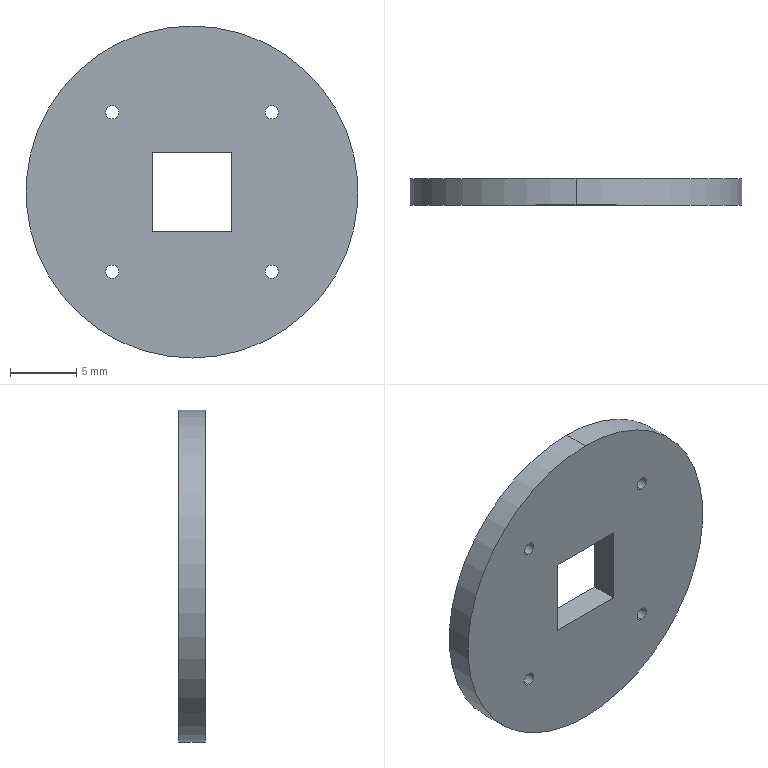Part | SolidWorks | features Extrusion 1 | 1 solid | 16 faces | box 25 x 2 x 25 mm | volume 903.465 mm3 | cylinder 10 | plane 6 | commonest cylinder face diameters 1 x8 25 x2
STEP:
#1=CARTESIAN_POINT('',(6.,2.,5.5));
#2=VERTEX_POINT('',#1);
#3=CARTESIAN_POINT('',(6.,2.,6.5));
#4=VERTEX_POINT('',#3);
#5=CARTESIAN_POINT('',(6.,2.,6.));
#6=DIRECTION('',(0.,1.,0.));
#7=DIRECTION('',(0.,0.,1.));
#8=AXIS2_PLACEMENT_3D('',#5,#6,#7);
#9=CIRCLE('',#8,0.5);
#10=EDGE_CURVE('',#2,#4,#9,.T.);
#11=ORIENTED_EDGE('',*,*,#10,.T.);
#12=CARTESIAN_POINT('',(6.,0.,6.5));
#13=VERTEX_POINT('',#12);
#14=CARTESIAN_POINT('',(6.,2.,6.5));
#15=DIRECTION('',(0.,-1.,0.));
#16=VECTOR('',#15,1000.);
#17=LINE('',#14,#16);
#18=EDGE_CURVE('',#4,#13,#17,.T.);
#19=ORIENTED_EDGE('',*,*,#18,.T.);
#20=CARTESIAN_POINT('',(6.,0.,5.5));
#21=VERTEX_POINT('',#20);
#22=CARTESIAN_POINT('',(6.,0.,6.));
#23=DIRECTION('',(0.,1.,0.));
#24=DIRECTION('',(0.,0.,1.));
#25=AXIS2_PLACEMENT_3D('',#22,#23,#24);
#26=CIRCLE('',#25,0.5);
#27=EDGE_CURVE('',#21,#13,#26,.T.);
#28=ORIENTED_EDGE('',*,*,#27,.F.);
#29=CARTESIAN_POINT('',(6.,2.,5.5));
#30=DIRECTION('',(0.,-1.,0.));
#31=VECTOR('',#30,1000.);
#32=LINE('',#29,#31);
#33=EDGE_CURVE('',#2,#21,#32,.T.);
#34=ORIENTED_EDGE('',*,*,#33,.F.);
#35=EDGE_LOOP('',(#11,#19,#28,#34));
#36=FACE_OUTER_BOUND('',#35,.T.);
#37=CARTESIAN_POINT('',(6.,2.,6.));
#38=DIRECTION('',(0.,-1.,0.));
#39=DIRECTION('',(0.,0.,-1.));
#40=AXIS2_PLACEMENT_3D('',#37,#38,#39);
#41=CYLINDRICAL_SURFACE('',#40,0.5);
#42=ADVANCED_FACE('',(#36),#41,.F.);
#43=CARTESIAN_POINT('',(6.,2.,-6.5));
#44=VERTEX_POINT('',#43);
#45=CARTESIAN_POINT('',(6.,2.,-5.5));
#46=VERTEX_POINT('',#45);
#47=CARTESIAN_POINT('',(6.,2.,-6.));
#48=DIRECTION('',(0.,1.,0.));
#49=DIRECTION('',(0.,0.,1.));
#50=AXIS2_PLACEMENT_3D('',#47,#48,#49);
#51=CIRCLE('',#50,0.5);
#52=EDGE_CURVE('',#44,#46,#51,.T.);
#53=ORIENTED_EDGE('',*,*,#52,.T.);
#54=CARTESIAN_POINT('',(6.,0.,-5.5));
#55=VERTEX_POINT('',#54);
#56=CARTESIAN_POINT('',(6.,2.,-5.5));
#57=DIRECTION('',(0.,-1.,0.));
#58=VECTOR('',#57,1000.);
#59=LINE('',#56,#58);
#60=EDGE_CURVE('',#46,#55,#59,.T.);
#61=ORIENTED_EDGE('',*,*,#60,.T.);
#62=CARTESIAN_POINT('',(6.,0.,-6.5));
#63=VERTEX_POINT('',#62);
#64=CARTESIAN_POINT('',(6.,0.,-6.));
#65=DIRECTION('',(0.,1.,0.));
#66=DIRECTION('',(0.,0.,1.));
#67=AXIS2_PLACEMENT_3D('',#64,#65,#66);
#68=CIRCLE('',#67,0.5);
#69=EDGE_CURVE('',#63,#55,#68,.T.);
#70=ORIENTED_EDGE('',*,*,#69,.F.);
#71=CARTESIAN_POINT('',(6.,2.,-6.5));
#72=DIRECTION('',(0.,-1.,0.));
#73=VECTOR('',#72,1000.);
#74=LINE('',#71,#73);
#75=EDGE_CURVE('',#44,#63,#74,.T.);
#76=ORIENTED_EDGE('',*,*,#75,.F.);
#77=EDGE_LOOP('',(#53,#61,#70,#76));
#78=FACE_OUTER_BOUND('',#77,.T.);
#79=CARTESIAN_POINT('',(6.,2.,-6.));
#80=DIRECTION('',(0.,-1.,0.));
#81=DIRECTION('',(0.,0.,-1.));
#82=AXIS2_PLACEMENT_3D('',#79,#80,#81);
#83=CYLINDRICAL_SURFACE('',#82,0.5);
#84=ADVANCED_FACE('',(#78),#83,.F.);
#85=CARTESIAN_POINT('',(-6.,2.,5.5));
#86=VERTEX_POINT('',#85);
#87=CARTESIAN_POINT('',(-6.,2.,6.5));
#88=VERTEX_POINT('',#87);
#89=CARTESIAN_POINT('',(-6.,2.,6.));
#90=DIRECTION('',(0.,1.,0.));
#91=DIRECTION('',(0.,0.,1.));
#92=AXIS2_PLACEMENT_3D('',#89,#90,#91);
#93=CIRCLE('',#92,0.5);
#94=EDGE_CURVE('',#86,#88,#93,.T.);
#95=ORIENTED_EDGE('',*,*,#94,.T.);
#96=CARTESIAN_POINT('',(-6.,0.,6.5));
#97=VERTEX_POINT('',#96);
#98=CARTESIAN_POINT('',(-6.,2.,6.5));
#99=DIRECTION('',(0.,-1.,0.));
#100=VECTOR('',#99,1000.);
#101=LINE('',#98,#100);
#102=EDGE_CURVE('',#88,#97,#101,.T.);
#103=ORIENTED_EDGE('',*,*,#102,.T.);
#104=CARTESIAN_POINT('',(-6.,0.,5.5));
#105=VERTEX_POINT('',#104);
#106=CARTESIAN_POINT('',(-6.,0.,6.));
#107=DIRECTION('',(0.,1.,0.));
#108=DIRECTION('',(0.,0.,1.));
#109=AXIS2_PLACEMENT_3D('',#106,#107,#108);
#110=CIRCLE('',#109,0.5);
#111=EDGE_CURVE('',#105,#97,#110,.T.);
#112=ORIENTED_EDGE('',*,*,#111,.F.);
#113=CARTESIAN_POINT('',(-6.,2.,5.5));
#114=DIRECTION('',(0.,-1.,0.));
#115=VECTOR('',#114,1000.);
#116=LINE('',#113,#115);
#117=EDGE_CURVE('',#86,#105,#116,.T.);
#118=ORIENTED_EDGE('',*,*,#117,.F.);
#119=EDGE_LOOP('',(#95,#103,#112,#118));
#120=FACE_OUTER_BOUND('',#119,.T.);
#121=CARTESIAN_POINT('',(-6.,2.,6.));
#122=DIRECTION('',(0.,-1.,0.));
#123=DIRECTION('',(0.,0.,-1.));
#124=AXIS2_PLACEMENT_3D('',#121,#122,#123);
#125=CYLINDRICAL_SURFACE('',#124,0.5);
#126=ADVANCED_FACE('',(#120),#125,.F.);
#127=CARTESIAN_POINT('',(-6.,2.,-6.5));
#128=VERTEX_POINT('',#127);
#129=CARTESIAN_POINT('',(-6.,2.,-5.5));
#130=VERTEX_POINT('',#129);
#131=CARTESIAN_POINT('',(-6.,2.,-6.));
#132=DIRECTION('',(0.,1.,0.));
#133=DIRECTION('',(0.,0.,1.));
#134=AXIS2_PLACEMENT_3D('',#131,#132,#133);
#135=CIRCLE('',#134,0.5);
#136=EDGE_CURVE('',#128,#130,#135,.T.);
#137=ORIENTED_EDGE('',*,*,#136,.T.);
#138=CARTESIAN_POINT('',(-6.,0.,-5.5));
#139=VERTEX_POINT('',#138);
#140=CARTESIAN_POINT('',(-6.,2.,-5.5));
#141=DIRECTION('',(0.,-1.,0.));
#142=VECTOR('',#141,1000.);
#143=LINE('',#140,#142);
#144=EDGE_CURVE('',#130,#139,#143,.T.);
#145=ORIENTED_EDGE('',*,*,#144,.T.);
#146=CARTESIAN_POINT('',(-6.,0.,-6.5));
#147=VERTEX_POINT('',#146);
#148=CARTESIAN_POINT('',(-6.,0.,-6.));
#149=DIRECTION('',(0.,1.,0.));
#150=DIRECTION('',(0.,0.,1.));
#151=AXIS2_PLACEMENT_3D('',#148,#149,#150);
#152=CIRCLE('',#151,0.5);
#153=EDGE_CURVE('',#147,#139,#152,.T.);
#154=ORIENTED_EDGE('',*,*,#153,.F.);
#155=CARTESIAN_POINT('',(-6.,2.,-6.5));
#156=DIRECTION('',(0.,-1.,0.));
#157=VECTOR('',#156,1000.);
#158=LINE('',#155,#157);
#159=EDGE_CURVE('',#128,#147,#158,.T.);
#160=ORIENTED_EDGE('',*,*,#159,.F.);
#161=EDGE_LOOP('',(#137,#145,#154,#160));
#162=FACE_OUTER_BOUND('',#161,.T.);
#163=CARTESIAN_POINT('',(-6.,2.,-6.));
#164=DIRECTION('',(0.,-1.,0.));
#165=DIRECTION('',(0.,0.,-1.));
#166=AXIS2_PLACEMENT_3D('',#163,#164,#165);
#167=CYLINDRICAL_SURFACE('',#166,0.5);
#168=ADVANCED_FACE('',(#162),#167,.F.);
#169=CARTESIAN_POINT('',(0.,2.,12.5));
#170=VERTEX_POINT('',#169);
#171=CARTESIAN_POINT('',(0.,2.,-12.5));
#172=VERTEX_POINT('',#171);
#173=CARTESIAN_POINT('',(0.,2.,0.));
#174=DIRECTION('',(0.,1.,0.));
#175=DIRECTION('',(0.,0.,1.));
#176=AXIS2_PLACEMENT_3D('',#173,#174,#175);
#177=CIRCLE('',#176,12.5);
#178=EDGE_CURVE('',#170,#172,#177,.T.);
#179=ORIENTED_EDGE('',*,*,#178,.F.);
#180=CARTESIAN_POINT('',(0.,0.,12.5));
#181=VERTEX_POINT('',#180);
#182=CARTESIAN_POINT('',(0.,2.,12.5));
#183=DIRECTION('',(0.,-1.,0.));
#184=VECTOR('',#183,1000.);
#185=LINE('',#182,#184);
#186=EDGE_CURVE('',#170,#181,#185,.T.);
#187=ORIENTED_EDGE('',*,*,#186,.T.);
#188=CARTESIAN_POINT('',(0.,0.,-12.5));
#189=VERTEX_POINT('',#188);
#190=CARTESIAN_POINT('',(0.,0.,0.));
#191=DIRECTION('',(0.,1.,0.));
#192=DIRECTION('',(0.,0.,1.));
#193=AXIS2_PLACEMENT_3D('',#190,#191,#192);
#194=CIRCLE('',#193,12.5);
#195=EDGE_CURVE('',#181,#189,#194,.T.);
#196=ORIENTED_EDGE('',*,*,#195,.T.);
#197=CARTESIAN_POINT('',(0.,2.,-12.5));
#198=DIRECTION('',(0.,-1.,0.));
#199=VECTOR('',#198,1000.);
#200=LINE('',#197,#199);
#201=EDGE_CURVE('',#172,#189,#200,.T.);
#202=ORIENTED_EDGE('',*,*,#201,.F.);
#203=EDGE_LOOP('',(#179,#187,#196,#202));
#204=FACE_OUTER_BOUND('',#203,.T.);
#205=CARTESIAN_POINT('',(0.,2.,0.));
#206=DIRECTION('',(0.,-1.,0.));
#207=DIRECTION('',(0.,0.,-1.));
#208=AXIS2_PLACEMENT_3D('',#205,#206,#207);
#209=CYLINDRICAL_SURFACE('',#208,12.5);
#210=ADVANCED_FACE('',(#204),#209,.T.);
#211=ORIENTED_EDGE('',*,*,#52,.F.);
#212=CARTESIAN_POINT('',(6.,2.,-6.));
#213=DIRECTION('',(0.,1.,0.));
#214=DIRECTION('',(0.,0.,1.));
#215=AXIS2_PLACEMENT_3D('',#212,#213,#214);
#216=CIRCLE('',#215,0.5);
#217=EDGE_CURVE('',#46,#44,#216,.T.);
#218=ORIENTED_EDGE('',*,*,#217,.F.);
#219=EDGE_LOOP('',(#211,#218));
#220=FACE_BOUND('',#219,.T.);
#221=ORIENTED_EDGE('',*,*,#136,.F.);
#222=CARTESIAN_POINT('',(-6.,2.,-6.));
#223=DIRECTION('',(0.,1.,0.));
#224=DIRECTION('',(0.,0.,1.));
#225=AXIS2_PLACEMENT_3D('',#222,#223,#224);
#226=CIRCLE('',#225,0.5);
#227=EDGE_CURVE('',#130,#128,#226,.T.);
#228=ORIENTED_EDGE('',*,*,#227,.F.);
#229=EDGE_LOOP('',(#221,#228));
#230=FACE_BOUND('',#229,.T.);
#231=CARTESIAN_POINT('',(0.,2.,0.));
#232=DIRECTION('',(0.,1.,0.));
#233=DIRECTION('',(0.,0.,1.));
#234=AXIS2_PLACEMENT_3D('',#231,#232,#233);
#235=CIRCLE('',#234,12.5);
#236=EDGE_CURVE('',#172,#170,#235,.T.);
#237=ORIENTED_EDGE('',*,*,#236,.T.);
#238=ORIENTED_EDGE('',*,*,#178,.T.);
#239=EDGE_LOOP('',(#237,#238));
#240=FACE_OUTER_BOUND('',#239,.T.);
#241=CARTESIAN_POINT('',(3.,2.,-3.));
#242=VERTEX_POINT('',#241);
#243=CARTESIAN_POINT('',(-3.,2.,-3.));
#244=VERTEX_POINT('',#243);
#245=CARTESIAN_POINT('',(3.,2.,-3.));
#246=DIRECTION('',(-1.,0.,0.));
#247=VECTOR('',#246,1000.);
#248=LINE('',#245,#247);
#249=EDGE_CURVE('',#242,#244,#248,.T.);
#250=ORIENTED_EDGE('',*,*,#249,.F.);
#251=CARTESIAN_POINT('',(3.,2.,3.));
#252=VERTEX_POINT('',#251);
#253=CARTESIAN_POINT('',(3.,2.,3.));
#254=DIRECTION('',(0.,0.,-1.));
#255=VECTOR('',#254,1000.);
#256=LINE('',#253,#255);
#257=EDGE_CURVE('',#252,#242,#256,.T.);
#258=ORIENTED_EDGE('',*,*,#257,.F.);
#259=CARTESIAN_POINT('',(-3.,2.,3.));
#260=VERTEX_POINT('',#259);
#261=CARTESIAN_POINT('',(-3.,2.,3.));
#262=DIRECTION('',(1.,0.,0.));
#263=VECTOR('',#262,1000.);
#264=LINE('',#261,#263);
#265=EDGE_CURVE('',#260,#252,#264,.T.);
#266=ORIENTED_EDGE('',*,*,#265,.F.);
#267=CARTESIAN_POINT('',(-3.,2.,-3.));
#268=DIRECTION('',(0.,0.,1.));
#269=VECTOR('',#268,1000.);
#270=LINE('',#267,#269);
#271=EDGE_CURVE('',#244,#260,#270,.T.);
#272=ORIENTED_EDGE('',*,*,#271,.F.);
#273=EDGE_LOOP('',(#250,#258,#266,#272));
#274=FACE_BOUND('',#273,.T.);
#275=ORIENTED_EDGE('',*,*,#94,.F.);
#276=CARTESIAN_POINT('',(-6.,2.,6.));
#277=DIRECTION('',(0.,1.,0.));
#278=DIRECTION('',(0.,0.,1.));
#279=AXIS2_PLACEMENT_3D('',#276,#277,#278);
#280=CIRCLE('',#279,0.5);
#281=EDGE_CURVE('',#88,#86,#280,.T.);
#282=ORIENTED_EDGE('',*,*,#281,.F.);
#283=EDGE_LOOP('',(#275,#282));
#284=FACE_BOUND('',#283,.T.);
#285=ORIENTED_EDGE('',*,*,#10,.F.);
#286=CARTESIAN_POINT('',(6.,2.,6.));
#287=DIRECTION('',(0.,1.,0.));
#288=DIRECTION('',(0.,0.,1.));
#289=AXIS2_PLACEMENT_3D('',#286,#287,#288);
#290=CIRCLE('',#289,0.5);
#291=EDGE_CURVE('',#4,#2,#290,.T.);
#292=ORIENTED_EDGE('',*,*,#291,.F.);
#293=EDGE_LOOP('',(#285,#292));
#294=FACE_BOUND('',#293,.T.);
#295=CARTESIAN_POINT('',(0.,2.,0.));
#296=DIRECTION('',(0.,1.,0.));
#297=DIRECTION('',(0.,0.,1.));
#298=AXIS2_PLACEMENT_3D('',#295,#296,#297);
#299=PLANE('',#298);
#300=ADVANCED_FACE('',(#220,#230,#240,#274,#284,#294),#299,.T.);
#301=CARTESIAN_POINT('',(0.,0.,0.));
#302=DIRECTION('',(0.,1.,0.));
#303=DIRECTION('',(0.,0.,1.));
#304=AXIS2_PLACEMENT_3D('',#301,#302,#303);
#305=CIRCLE('',#304,12.5);
#306=EDGE_CURVE('',#189,#181,#305,.T.);
#307=ORIENTED_EDGE('',*,*,#306,.F.);
#308=ORIENTED_EDGE('',*,*,#195,.F.);
#309=EDGE_LOOP('',(#307,#308));
#310=FACE_OUTER_BOUND('',#309,.T.);
#311=CARTESIAN_POINT('',(3.,0.,3.));
#312=VERTEX_POINT('',#311);
#313=CARTESIAN_POINT('',(3.,0.,-3.));
#314=VERTEX_POINT('',#313);
#315=CARTESIAN_POINT('',(3.,0.,3.));
#316=DIRECTION('',(0.,0.,-1.));
#317=VECTOR('',#316,1000.);
#318=LINE('',#315,#317);
#319=EDGE_CURVE('',#312,#314,#318,.T.);
#320=ORIENTED_EDGE('',*,*,#319,.T.);
#321=CARTESIAN_POINT('',(-3.,0.,-3.));
#322=VERTEX_POINT('',#321);
#323=CARTESIAN_POINT('',(3.,0.,-3.));
#324=DIRECTION('',(-1.,0.,0.));
#325=VECTOR('',#324,1000.);
#326=LINE('',#323,#325);
#327=EDGE_CURVE('',#314,#322,#326,.T.);
#328=ORIENTED_EDGE('',*,*,#327,.T.);
#329=CARTESIAN_POINT('',(-3.,0.,3.));
#330=VERTEX_POINT('',#329);
#331=CARTESIAN_POINT('',(-3.,0.,-3.));
#332=DIRECTION('',(0.,0.,1.));
#333=VECTOR('',#332,1000.);
#334=LINE('',#331,#333);
#335=EDGE_CURVE('',#322,#330,#334,.T.);
#336=ORIENTED_EDGE('',*,*,#335,.T.);
#337=CARTESIAN_POINT('',(-3.,0.,3.));
#338=DIRECTION('',(1.,0.,0.));
#339=VECTOR('',#338,1000.);
#340=LINE('',#337,#339);
#341=EDGE_CURVE('',#330,#312,#340,.T.);
#342=ORIENTED_EDGE('',*,*,#341,.T.);
#343=EDGE_LOOP('',(#320,#328,#336,#342));
#344=FACE_BOUND('',#343,.T.);
#345=ORIENTED_EDGE('',*,*,#153,.T.);
#346=CARTESIAN_POINT('',(-6.,0.,-6.));
#347=DIRECTION('',(0.,1.,0.));
#348=DIRECTION('',(0.,0.,1.));
#349=AXIS2_PLACEMENT_3D('',#346,#347,#348);
#350=CIRCLE('',#349,0.5);
#351=EDGE_CURVE('',#139,#147,#350,.T.);
#352=ORIENTED_EDGE('',*,*,#351,.T.);
#353=EDGE_LOOP('',(#345,#352));
#354=FACE_BOUND('',#353,.T.);
#355=ORIENTED_EDGE('',*,*,#111,.T.);
#356=CARTESIAN_POINT('',(-6.,0.,6.));
#357=DIRECTION('',(0.,1.,0.));
#358=DIRECTION('',(0.,0.,1.));
#359=AXIS2_PLACEMENT_3D('',#356,#357,#358);
#360=CIRCLE('',#359,0.5);
#361=EDGE_CURVE('',#97,#105,#360,.T.);
#362=ORIENTED_EDGE('',*,*,#361,.T.);
#363=EDGE_LOOP('',(#355,#362));
#364=FACE_BOUND('',#363,.T.);
#365=ORIENTED_EDGE('',*,*,#69,.T.);
#366=CARTESIAN_POINT('',(6.,0.,-6.));
#367=DIRECTION('',(0.,1.,0.));
#368=DIRECTION('',(0.,0.,1.));
#369=AXIS2_PLACEMENT_3D('',#366,#367,#368);
#370=CIRCLE('',#369,0.5);
#371=EDGE_CURVE('',#55,#63,#370,.T.);
#372=ORIENTED_EDGE('',*,*,#371,.T.);
#373=EDGE_LOOP('',(#365,#372));
#374=FACE_BOUND('',#373,.T.);
#375=ORIENTED_EDGE('',*,*,#27,.T.);
#376=CARTESIAN_POINT('',(6.,0.,6.));
#377=DIRECTION('',(0.,1.,0.));
#378=DIRECTION('',(0.,0.,1.));
#379=AXIS2_PLACEMENT_3D('',#376,#377,#378);
#380=CIRCLE('',#379,0.5);
#381=EDGE_CURVE('',#13,#21,#380,.T.);
#382=ORIENTED_EDGE('',*,*,#381,.T.);
#383=EDGE_LOOP('',(#375,#382));
#384=FACE_BOUND('',#383,.T.);
#385=CARTESIAN_POINT('',(0.,0.,0.));
#386=DIRECTION('',(0.,1.,0.));
#387=DIRECTION('',(0.,0.,1.));
#388=AXIS2_PLACEMENT_3D('',#385,#386,#387);
#389=PLANE('',#388);
#390=ADVANCED_FACE('',(#310,#344,#354,#364,#374,#384),#389,.F.);
#391=ORIENTED_EDGE('',*,*,#186,.F.);
#392=ORIENTED_EDGE('',*,*,#236,.F.);
#393=ORIENTED_EDGE('',*,*,#201,.T.);
#394=ORIENTED_EDGE('',*,*,#306,.T.);
#395=EDGE_LOOP('',(#391,#392,#393,#394));
#396=FACE_OUTER_BOUND('',#395,.T.);
#397=CARTESIAN_POINT('',(0.,2.,0.));
#398=DIRECTION('',(0.,-1.,0.));
#399=DIRECTION('',(0.,0.,-1.));
#400=AXIS2_PLACEMENT_3D('',#397,#398,#399);
#401=CYLINDRICAL_SURFACE('',#400,12.5);
#402=ADVANCED_FACE('',(#396),#401,.T.);
#403=ORIENTED_EDGE('',*,*,#319,.F.);
#404=CARTESIAN_POINT('',(3.,2.,3.));
#405=DIRECTION('',(0.,-1.,0.));
#406=VECTOR('',#405,1000.);
#407=LINE('',#404,#406);
#408=EDGE_CURVE('',#252,#312,#407,.T.);
#409=ORIENTED_EDGE('',*,*,#408,.F.);
#410=ORIENTED_EDGE('',*,*,#257,.T.);
#411=CARTESIAN_POINT('',(3.,2.,-3.));
#412=DIRECTION('',(0.,-1.,0.));
#413=VECTOR('',#412,1000.);
#414=LINE('',#411,#413);
#415=EDGE_CURVE('',#242,#314,#414,.T.);
#416=ORIENTED_EDGE('',*,*,#415,.T.);
#417=EDGE_LOOP('',(#403,#409,#410,#416));
#418=FACE_OUTER_BOUND('',#417,.T.);
#419=CARTESIAN_POINT('',(3.,2.,3.));
#420=DIRECTION('',(-1.,0.,0.));
#421=DIRECTION('',(0.,0.,1.));
#422=AXIS2_PLACEMENT_3D('',#419,#420,#421);
#423=PLANE('',#422);
#424=ADVANCED_FACE('',(#418),#423,.T.);
#425=ORIENTED_EDGE('',*,*,#327,.F.);
#426=ORIENTED_EDGE('',*,*,#415,.F.);
#427=ORIENTED_EDGE('',*,*,#249,.T.);
#428=CARTESIAN_POINT('',(-3.,2.,-3.));
#429=DIRECTION('',(0.,-1.,0.));
#430=VECTOR('',#429,1000.);
#431=LINE('',#428,#430);
#432=EDGE_CURVE('',#244,#322,#431,.T.);
#433=ORIENTED_EDGE('',*,*,#432,.T.);
#434=EDGE_LOOP('',(#425,#426,#427,#433));
#435=FACE_OUTER_BOUND('',#434,.T.);
#436=CARTESIAN_POINT('',(3.,2.,-3.));
#437=DIRECTION('',(0.,0.,1.));
#438=DIRECTION('',(1.,0.,0.));
#439=AXIS2_PLACEMENT_3D('',#436,#437,#438);
#440=PLANE('',#439);
#441=ADVANCED_FACE('',(#435),#440,.T.);
#442=ORIENTED_EDGE('',*,*,#335,.F.);
#443=ORIENTED_EDGE('',*,*,#432,.F.);
#444=ORIENTED_EDGE('',*,*,#271,.T.);
#445=CARTESIAN_POINT('',(-3.,2.,3.));
#446=DIRECTION('',(0.,-1.,0.));
#447=VECTOR('',#446,1000.);
#448=LINE('',#445,#447);
#449=EDGE_CURVE('',#260,#330,#448,.T.);
#450=ORIENTED_EDGE('',*,*,#449,.T.);
#451=EDGE_LOOP('',(#442,#443,#444,#450));
#452=FACE_OUTER_BOUND('',#451,.T.);
#453=CARTESIAN_POINT('',(-3.,2.,-3.));
#454=DIRECTION('',(1.,0.,0.));
#455=DIRECTION('',(0.,0.,-1.));
#456=AXIS2_PLACEMENT_3D('',#453,#454,#455);
#457=PLANE('',#456);
#458=ADVANCED_FACE('',(#452),#457,.T.);
#459=ORIENTED_EDGE('',*,*,#341,.F.);
#460=ORIENTED_EDGE('',*,*,#449,.F.);
#461=ORIENTED_EDGE('',*,*,#265,.T.);
#462=ORIENTED_EDGE('',*,*,#408,.T.);
#463=EDGE_LOOP('',(#459,#460,#461,#462));
#464=FACE_OUTER_BOUND('',#463,.T.);
#465=CARTESIAN_POINT('',(-3.,2.,3.));
#466=DIRECTION('',(0.,0.,-1.));
#467=DIRECTION('',(-1.,0.,0.));
#468=AXIS2_PLACEMENT_3D('',#465,#466,#467);
#469=PLANE('',#468);
#470=ADVANCED_FACE('',(#464),#469,.T.);
#471=ORIENTED_EDGE('',*,*,#144,.F.);
#472=ORIENTED_EDGE('',*,*,#227,.T.);
#473=ORIENTED_EDGE('',*,*,#159,.T.);
#474=ORIENTED_EDGE('',*,*,#351,.F.);
#475=EDGE_LOOP('',(#471,#472,#473,#474));
#476=FACE_OUTER_BOUND('',#475,.T.);
#477=CARTESIAN_POINT('',(-6.,2.,-6.));
#478=DIRECTION('',(0.,-1.,0.));
#479=DIRECTION('',(0.,0.,-1.));
#480=AXIS2_PLACEMENT_3D('',#477,#478,#479);
#481=CYLINDRICAL_SURFACE('',#480,0.5);
#482=ADVANCED_FACE('',(#476),#481,.F.);
#483=ORIENTED_EDGE('',*,*,#102,.F.);
#484=ORIENTED_EDGE('',*,*,#281,.T.);
#485=ORIENTED_EDGE('',*,*,#117,.T.);
#486=ORIENTED_EDGE('',*,*,#361,.F.);
#487=EDGE_LOOP('',(#483,#484,#485,#486));
#488=FACE_OUTER_BOUND('',#487,.T.);
#489=CARTESIAN_POINT('',(-6.,2.,6.));
#490=DIRECTION('',(0.,-1.,0.));
#491=DIRECTION('',(0.,0.,-1.));
#492=AXIS2_PLACEMENT_3D('',#489,#490,#491);
#493=CYLINDRICAL_SURFACE('',#492,0.5);
#494=ADVANCED_FACE('',(#488),#493,.F.);
#495=ORIENTED_EDGE('',*,*,#60,.F.);
#496=ORIENTED_EDGE('',*,*,#217,.T.);
#497=ORIENTED_EDGE('',*,*,#75,.T.);
#498=ORIENTED_EDGE('',*,*,#371,.F.);
#499=EDGE_LOOP('',(#495,#496,#497,#498));
#500=FACE_OUTER_BOUND('',#499,.T.);
#501=CARTESIAN_POINT('',(6.,2.,-6.));
#502=DIRECTION('',(0.,-1.,0.));
#503=DIRECTION('',(0.,0.,-1.));
#504=AXIS2_PLACEMENT_3D('',#501,#502,#503);
#505=CYLINDRICAL_SURFACE('',#504,0.5);
#506=ADVANCED_FACE('',(#500),#505,.F.);
#507=ORIENTED_EDGE('',*,*,#18,.F.);
#508=ORIENTED_EDGE('',*,*,#291,.T.);
#509=ORIENTED_EDGE('',*,*,#33,.T.);
#510=ORIENTED_EDGE('',*,*,#381,.F.);
#511=EDGE_LOOP('',(#507,#508,#509,#510));
#512=FACE_OUTER_BOUND('',#511,.T.);
#513=CARTESIAN_POINT('',(6.,2.,6.));
#514=DIRECTION('',(0.,-1.,0.));
#515=DIRECTION('',(0.,0.,-1.));
#516=AXIS2_PLACEMENT_3D('',#513,#514,#515);
#517=CYLINDRICAL_SURFACE('',#516,0.5);
#518=ADVANCED_FACE('',(#512),#517,.F.);
#519=CLOSED_SHELL('',(#42,#84,#126,#168,#210,#300,#390,#402,#424,#441,#458,#470,#482,#494,#506,#518));
#520=MANIFOLD_SOLID_BREP('',#519);
#521=CARTESIAN_POINT('',(0.,0.,0.));
#522=DIRECTION('',(0.,0.,1.));
#523=DIRECTION('',(1.,0.,0.));
#524=AXIS2_PLACEMENT_3D('',#521,#522,#523);
#525=(LENGTH_UNIT()NAMED_UNIT(*)SI_UNIT(.MILLI.,.METRE.));
#526=UNCERTAINTY_MEASURE_WITH_UNIT(LENGTH_MEASURE(0.00001),#525,'','');
#527=(NAMED_UNIT(*)PLANE_ANGLE_UNIT()SI_UNIT($,.RADIAN.));
#528=(NAMED_UNIT(*)SI_UNIT($,.STERADIAN.)SOLID_ANGLE_UNIT());
#529=(GEOMETRIC_REPRESENTATION_CONTEXT(3)GLOBAL_UNCERTAINTY_ASSIGNED_CONTEXT((#526))GLOBAL_UNIT_ASSIGNED_CONTEXT((#525,#527,#528))REPRESENTATION_CONTEXT('',''));
#530=ADVANCED_BREP_SHAPE_REPRESENTATION('',(#520,#524),#529);